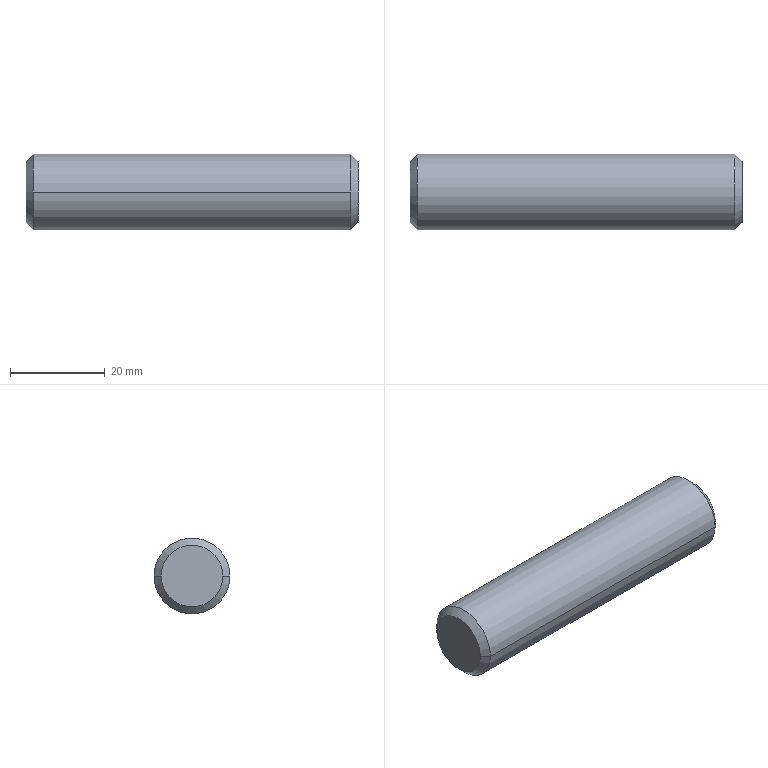Part | SolidWorks | features Revolution 1 | 1 solid | 8 faces | box 70 x 16 x 16 mm | volume 13968 mm3 | cone 4 | cylinder 2 | plane 2 | commonest cylinder face diameters 16 x2
STEP:
#1=CARTESIAN_POINT('',(0.,14.5,0.));
#2=VERTEX_POINT('',#1);
#3=CARTESIAN_POINT('',(0.,1.5,0.));
#4=VERTEX_POINT('',#3);
#5=CARTESIAN_POINT('',(0.,8.,0.));
#6=DIRECTION('',(1.,0.,0.));
#7=DIRECTION('',(0.,1.,0.));
#8=AXIS2_PLACEMENT_3D('',#5,#6,#7);
#9=CIRCLE('',#8,6.5);
#10=EDGE_CURVE('',#2,#4,#9,.T.);
#11=ORIENTED_EDGE('',*,*,#10,.F.);
#12=CARTESIAN_POINT('',(-1.5,16.,0.));
#13=VERTEX_POINT('',#12);
#14=CARTESIAN_POINT('',(0.,14.5,0.));
#15=DIRECTION('',(-0.7071,0.7071,0.));
#16=VECTOR('',#15,1000.);
#17=LINE('',#14,#16);
#18=EDGE_CURVE('',#2,#13,#17,.T.);
#19=ORIENTED_EDGE('',*,*,#18,.T.);
#20=CARTESIAN_POINT('',(-1.5,0.,0.));
#21=VERTEX_POINT('',#20);
#22=CARTESIAN_POINT('',(-1.5,8.,0.));
#23=DIRECTION('',(1.,0.,0.));
#24=DIRECTION('',(0.,1.,0.));
#25=AXIS2_PLACEMENT_3D('',#22,#23,#24);
#26=CIRCLE('',#25,8.);
#27=EDGE_CURVE('',#13,#21,#26,.T.);
#28=ORIENTED_EDGE('',*,*,#27,.T.);
#29=CARTESIAN_POINT('',(0.,1.5,0.));
#30=DIRECTION('',(-0.7071,-0.7071,0.));
#31=VECTOR('',#30,1000.);
#32=LINE('',#29,#31);
#33=EDGE_CURVE('',#4,#21,#32,.T.);
#34=ORIENTED_EDGE('',*,*,#33,.F.);
#35=EDGE_LOOP('',(#11,#19,#28,#34));
#36=FACE_OUTER_BOUND('',#35,.T.);
#37=CARTESIAN_POINT('',(0.,8.,0.));
#38=DIRECTION('',(-1.,0.,0.));
#39=DIRECTION('',(0.,-1.,0.));
#40=AXIS2_PLACEMENT_3D('',#37,#38,#39);
#41=CONICAL_SURFACE('',#40,6.5,0.7854);
#42=ADVANCED_FACE('',(#36),#41,.T.);
#43=CARTESIAN_POINT('',(-68.5,16.,0.));
#44=VERTEX_POINT('',#43);
#45=CARTESIAN_POINT('',(-68.5,0.,0.));
#46=VERTEX_POINT('',#45);
#47=CARTESIAN_POINT('',(-68.5,8.,0.));
#48=DIRECTION('',(1.,0.,0.));
#49=DIRECTION('',(0.,1.,0.));
#50=AXIS2_PLACEMENT_3D('',#47,#48,#49);
#51=CIRCLE('',#50,8.);
#52=EDGE_CURVE('',#44,#46,#51,.T.);
#53=ORIENTED_EDGE('',*,*,#52,.T.);
#54=CARTESIAN_POINT('',(-70.,0.,0.));
#55=DIRECTION('',(1.,0.,0.));
#56=VECTOR('',#55,1000.);
#57=LINE('',#54,#56);
#58=EDGE_CURVE('',#46,#21,#57,.T.);
#59=ORIENTED_EDGE('',*,*,#58,.T.);
#60=ORIENTED_EDGE('',*,*,#27,.F.);
#61=CARTESIAN_POINT('',(-70.,16.,0.));
#62=DIRECTION('',(1.,0.,0.));
#63=VECTOR('',#62,1000.);
#64=LINE('',#61,#63);
#65=EDGE_CURVE('',#44,#13,#64,.T.);
#66=ORIENTED_EDGE('',*,*,#65,.F.);
#67=EDGE_LOOP('',(#53,#59,#60,#66));
#68=FACE_OUTER_BOUND('',#67,.T.);
#69=CARTESIAN_POINT('',(-70.,8.,0.));
#70=DIRECTION('',(1.,0.,0.));
#71=DIRECTION('',(0.,1.,0.));
#72=AXIS2_PLACEMENT_3D('',#69,#70,#71);
#73=CYLINDRICAL_SURFACE('',#72,8.);
#74=ADVANCED_FACE('',(#68),#73,.T.);
#75=CARTESIAN_POINT('',(-70.,14.5,0.));
#76=VERTEX_POINT('',#75);
#77=CARTESIAN_POINT('',(-70.,1.5,0.));
#78=VERTEX_POINT('',#77);
#79=CARTESIAN_POINT('',(-70.,8.,0.));
#80=DIRECTION('',(1.,0.,0.));
#81=DIRECTION('',(0.,1.,0.));
#82=AXIS2_PLACEMENT_3D('',#79,#80,#81);
#83=CIRCLE('',#82,6.5);
#84=EDGE_CURVE('',#76,#78,#83,.T.);
#85=ORIENTED_EDGE('',*,*,#84,.T.);
#86=CARTESIAN_POINT('',(-68.5,0.,0.));
#87=DIRECTION('',(0.7071,-0.7071,0.));
#88=VECTOR('',#87,1000.);
#89=LINE('',#86,#88);
#90=EDGE_CURVE('',#78,#46,#89,.T.);
#91=ORIENTED_EDGE('',*,*,#90,.T.);
#92=ORIENTED_EDGE('',*,*,#52,.F.);
#93=CARTESIAN_POINT('',(-68.5,16.,0.));
#94=DIRECTION('',(0.7071,0.7071,0.));
#95=VECTOR('',#94,1000.);
#96=LINE('',#93,#95);
#97=EDGE_CURVE('',#76,#44,#96,.T.);
#98=ORIENTED_EDGE('',*,*,#97,.F.);
#99=EDGE_LOOP('',(#85,#91,#92,#98));
#100=FACE_OUTER_BOUND('',#99,.T.);
#101=CARTESIAN_POINT('',(-68.5,8.,0.));
#102=DIRECTION('',(1.,0.,0.));
#103=DIRECTION('',(0.,1.,0.));
#104=AXIS2_PLACEMENT_3D('',#101,#102,#103);
#105=CONICAL_SURFACE('',#104,8.,0.7854);
#106=ADVANCED_FACE('',(#100),#105,.T.);
#107=ORIENTED_EDGE('',*,*,#90,.F.);
#108=CARTESIAN_POINT('',(-70.,8.,0.));
#109=DIRECTION('',(1.,0.,0.));
#110=DIRECTION('',(0.,1.,0.));
#111=AXIS2_PLACEMENT_3D('',#108,#109,#110);
#112=CIRCLE('',#111,6.5);
#113=EDGE_CURVE('',#78,#76,#112,.T.);
#114=ORIENTED_EDGE('',*,*,#113,.T.);
#115=ORIENTED_EDGE('',*,*,#97,.T.);
#116=CARTESIAN_POINT('',(-68.5,8.,0.));
#117=DIRECTION('',(1.,0.,0.));
#118=DIRECTION('',(0.,1.,0.));
#119=AXIS2_PLACEMENT_3D('',#116,#117,#118);
#120=CIRCLE('',#119,8.);
#121=EDGE_CURVE('',#46,#44,#120,.T.);
#122=ORIENTED_EDGE('',*,*,#121,.F.);
#123=EDGE_LOOP('',(#107,#114,#115,#122));
#124=FACE_OUTER_BOUND('',#123,.T.);
#125=CARTESIAN_POINT('',(-68.5,8.,0.));
#126=DIRECTION('',(1.,0.,0.));
#127=DIRECTION('',(0.,1.,0.));
#128=AXIS2_PLACEMENT_3D('',#125,#126,#127);
#129=CONICAL_SURFACE('',#128,8.,0.7854);
#130=ADVANCED_FACE('',(#124),#129,.T.);
#131=ORIENTED_EDGE('',*,*,#58,.F.);
#132=ORIENTED_EDGE('',*,*,#121,.T.);
#133=ORIENTED_EDGE('',*,*,#65,.T.);
#134=CARTESIAN_POINT('',(-1.5,8.,0.));
#135=DIRECTION('',(1.,0.,0.));
#136=DIRECTION('',(0.,1.,0.));
#137=AXIS2_PLACEMENT_3D('',#134,#135,#136);
#138=CIRCLE('',#137,8.);
#139=EDGE_CURVE('',#21,#13,#138,.T.);
#140=ORIENTED_EDGE('',*,*,#139,.F.);
#141=EDGE_LOOP('',(#131,#132,#133,#140));
#142=FACE_OUTER_BOUND('',#141,.T.);
#143=CARTESIAN_POINT('',(-70.,8.,0.));
#144=DIRECTION('',(1.,0.,0.));
#145=DIRECTION('',(0.,1.,0.));
#146=AXIS2_PLACEMENT_3D('',#143,#144,#145);
#147=CYLINDRICAL_SURFACE('',#146,8.);
#148=ADVANCED_FACE('',(#142),#147,.T.);
#149=ORIENTED_EDGE('',*,*,#18,.F.);
#150=CARTESIAN_POINT('',(0.,8.,0.));
#151=DIRECTION('',(1.,0.,0.));
#152=DIRECTION('',(0.,1.,0.));
#153=AXIS2_PLACEMENT_3D('',#150,#151,#152);
#154=CIRCLE('',#153,6.5);
#155=EDGE_CURVE('',#4,#2,#154,.T.);
#156=ORIENTED_EDGE('',*,*,#155,.F.);
#157=ORIENTED_EDGE('',*,*,#33,.T.);
#158=ORIENTED_EDGE('',*,*,#139,.T.);
#159=EDGE_LOOP('',(#149,#156,#157,#158));
#160=FACE_OUTER_BOUND('',#159,.T.);
#161=CARTESIAN_POINT('',(0.,8.,0.));
#162=DIRECTION('',(-1.,0.,0.));
#163=DIRECTION('',(0.,-1.,0.));
#164=AXIS2_PLACEMENT_3D('',#161,#162,#163);
#165=CONICAL_SURFACE('',#164,6.5,0.7854);
#166=ADVANCED_FACE('',(#160),#165,.T.);
#167=ORIENTED_EDGE('',*,*,#155,.T.);
#168=ORIENTED_EDGE('',*,*,#10,.T.);
#169=EDGE_LOOP('',(#167,#168));
#170=FACE_OUTER_BOUND('',#169,.T.);
#171=CARTESIAN_POINT('',(0.,8.,0.));
#172=DIRECTION('',(1.,0.,0.));
#173=DIRECTION('',(0.,1.,0.));
#174=AXIS2_PLACEMENT_3D('',#171,#172,#173);
#175=PLANE('',#174);
#176=ADVANCED_FACE('',(#170),#175,.T.);
#177=ORIENTED_EDGE('',*,*,#84,.F.);
#178=ORIENTED_EDGE('',*,*,#113,.F.);
#179=EDGE_LOOP('',(#177,#178));
#180=FACE_OUTER_BOUND('',#179,.T.);
#181=CARTESIAN_POINT('',(-70.,14.5,0.));
#182=DIRECTION('',(-1.,0.,0.));
#183=DIRECTION('',(0.,-1.,0.));
#184=AXIS2_PLACEMENT_3D('',#181,#182,#183);
#185=PLANE('',#184);
#186=ADVANCED_FACE('',(#180),#185,.T.);
#187=CLOSED_SHELL('',(#42,#74,#106,#130,#148,#166,#176,#186));
#188=MANIFOLD_SOLID_BREP('',#187);
#189=CARTESIAN_POINT('',(0.,0.,0.));
#190=DIRECTION('',(0.,0.,1.));
#191=DIRECTION('',(1.,0.,0.));
#192=AXIS2_PLACEMENT_3D('',#189,#190,#191);
#193=(LENGTH_UNIT()NAMED_UNIT(*)SI_UNIT(.MILLI.,.METRE.));
#194=UNCERTAINTY_MEASURE_WITH_UNIT(LENGTH_MEASURE(0.00001),#193,'','');
#195=(NAMED_UNIT(*)PLANE_ANGLE_UNIT()SI_UNIT($,.RADIAN.));
#196=(NAMED_UNIT(*)SI_UNIT($,.STERADIAN.)SOLID_ANGLE_UNIT());
#197=(GEOMETRIC_REPRESENTATION_CONTEXT(3)GLOBAL_UNCERTAINTY_ASSIGNED_CONTEXT((#194))GLOBAL_UNIT_ASSIGNED_CONTEXT((#193,#195,#196))REPRESENTATION_CONTEXT('',''));
#198=ADVANCED_BREP_SHAPE_REPRESENTATION('',(#188,#192),#197);